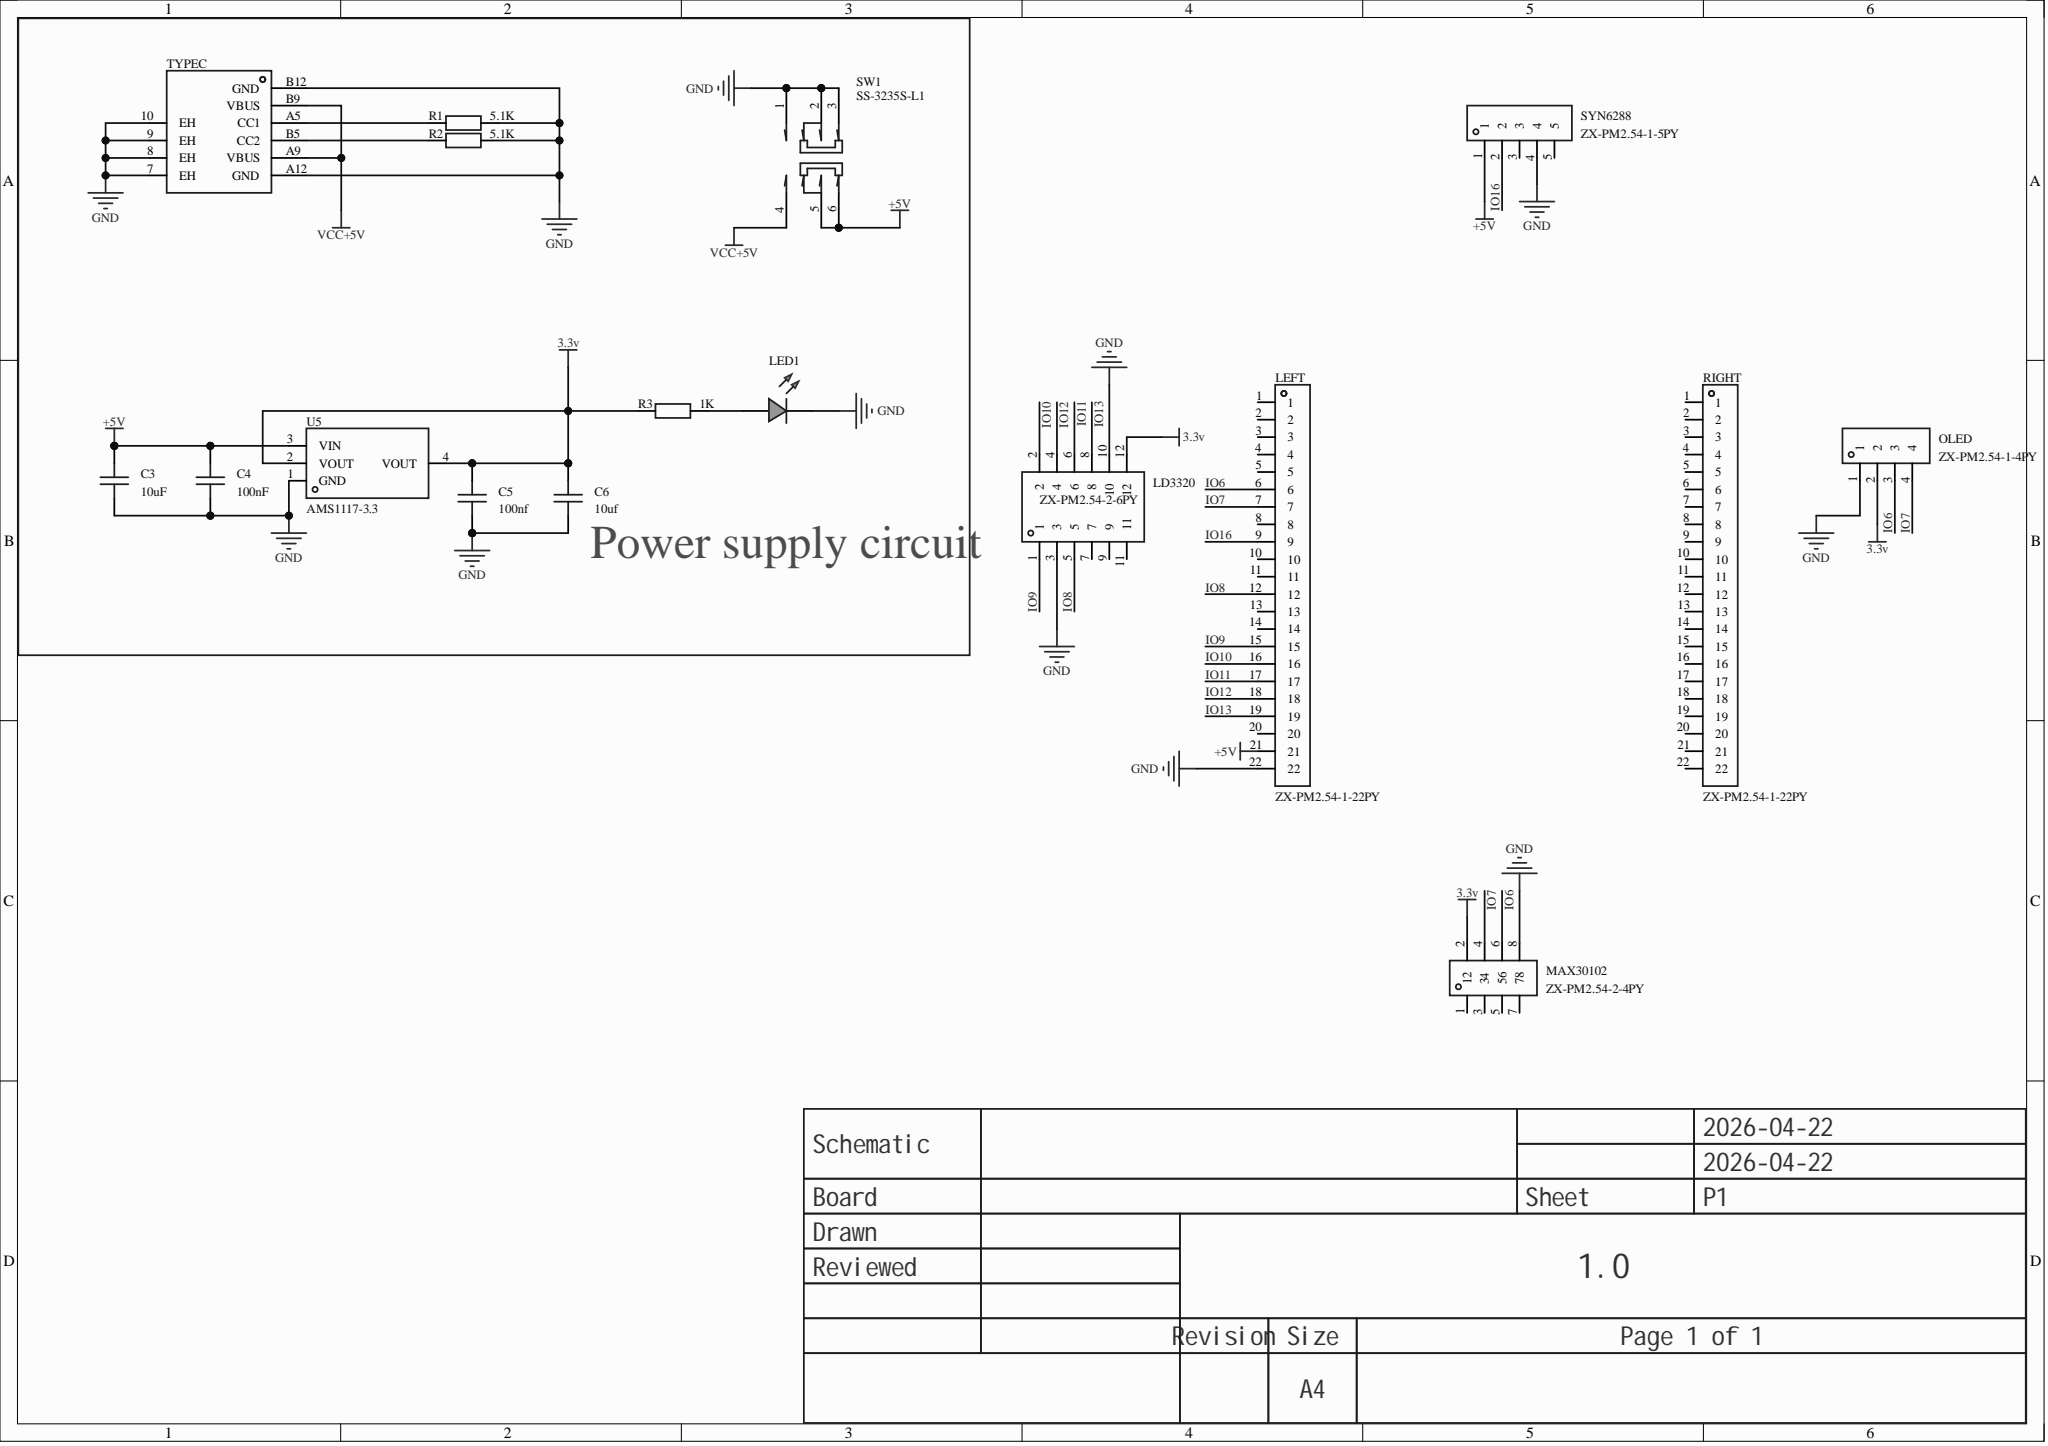Circuit board | Altium Designer | 17 parts | 16 nets
Bill of materials:
Comment,Description,Designator,Footprint,LibRef,Quantity
"10uF","Capacitance: 10uF; tolerance: ±20%; rated voltage: 25V; temperature coefficient: X5R;, [NoValue]","C3, C6","C0603","CL10A106MA8NRNC, CAP_0603","2"
"100nF","[NoValue], Capacitance: 10uF; tolerance: ±20%; rated voltage: 25V; temperature coefficient: X5R;","C4, C5","C0603","CAP_0603, CL10A106MA8NRNC","2"
"ZX-PM2.54-2-6PY","","LD3320","HDR-TH_12P-P2.54-V-F-R2-C6-S2.54","ZX-PM2.54-2-6PY","1"
"","","LED1","LED_0805","LED_0805-G","1"
"ZX-PM2.54-1-22PY","","LEFT, RIGHT","HDR-TH_22P-P2.54-V-F","ZX-PM2.54-1-22PY","2"
"ZX-PM2.54-2-4PY","","MAX30102","HDR-TH_8P-P2.54-V-F-R2-C4-S2.54","ZX-PM2.54-2-4PY","1"
"ZX-PM2.54-1-4PY","","OLED","HDR-TH_4P-P2.54-V-F","ZX-PM2.54-1-4PY","1"
"5.1K","","R1, R2","R0603","Res_0603","2"
"1K","","R3","R0603","Res_0603","1"
"SS-3235S-L1","","SW1","SW-SMD_SS-3235S-LX","SS-3235S-L1","1"
"ZX-PM2.54-1-5PY","","SYN6288","HDR-TH_5P-P2.54-V-F-B","ZX-PM2.54-1-5PY","1"
"","","TYPEC","USB_ TYPE-C-6P","USB_ Type-C-6P","1"
"AMS1117-3.3","Output type: fixed; working voltage: 15V; output voltage: 3.3V; output current: 1A; ripple rejection (PSRR): 72dB@(120Hz); output polarity: positive;","U5","SOT-223-3_L6.5-W3.4-P2.30-LS7.0-BR","AMS1117-3.3_C6186","1"
Netlist (Protel format):
[
C3
C0603
10uF



]
[
C4
C0603
100nF



]
[
C5
C0603
100nf



]
[
C6
C0603
10uf



]
[
LD3320
HDR-TH_12P-P2.54-V-F-R2-C6-S2.54
ZX-PM2.54-2-6PY



]
[
LED1
LED_0805




]
[
LEFT
HDR-TH_22P-P2.54-V-F
ZX-PM2.54-1-22PY



]
[
MAX30102
HDR-TH_8P-P2.54-V-F-R2-C4-S2.54
ZX-PM2.54-2-4PY



]
[
OLED
HDR-TH_4P-P2.54-V-F
ZX-PM2.54-1-4PY



]
[
R1
R0603
5.1K



]
[
R2
R0603
5.1K



]
[
R3
R0603
1K



]
[
RIGHT
HDR-TH_22P-P2.54-V-F
ZX-PM2.54-1-22PY



]
[
SW1
SW-SMD_SS-3235S-LX
SS-3235S-L1



]
[
SYN6288
HDR-TH_5P-P2.54-V-F-B
ZX-PM2.54-1-5PY



]
[
TYPEC
USB_ TYPE-C-6P




]
[
U5
SOT-223-3_L6.5-W3.4-P2.30-LS7.0-BR
AMS1117-3.3



]
(
VCC+5V
SW1-4
TYPEC-A9
TYPEC-B9
)
(
NetR2_1
R2-1
TYPEC-B5
)
(
NetR1_1
R1-1
TYPEC-A5
)
(
NetLED1_2
LED1-2
R3-2
)
(
IO16
LEFT-9
SYN6288-2
)
(
IO13
LD3320-8
LEFT-19
)
(
IO12
LD3320-4
LEFT-18
)
(
IO11
LD3320-6
LEFT-17
)
(
IO10
LD3320-2
LEFT-16
)
(
IO9
LD3320-1
LEFT-15
)
(
IO8
LD3320-5
LEFT-12
)
(
IO7
LEFT-7
MAX30102-4
OLED-4
)
(
IO6
LEFT-6
MAX30102-6
OLED-3
)
(
GND
C3-1
C4-1
C5-1
C6-1
LD3320-3
LD3320-10
LED1-1
LEFT-22
MAX30102-8
OLED-1
R1-2
R2-2
SW1-1
SW1-2
SW1-3
SYN6288-4
TYPEC-7
TYPEC-8
TYPEC-9
TYPEC-10
TYPEC-A12
TYPEC-B12
U5-1
)
(
+5V
C3-2
C4-2
LEFT-21
SW1-5
SW1-6
SYN6288-1
U5-3
)
(
3.3v
C5-2
C6-2
LD3320-12
MAX30102-2
OLED-2
R3-1
U5-2
U5-4
)